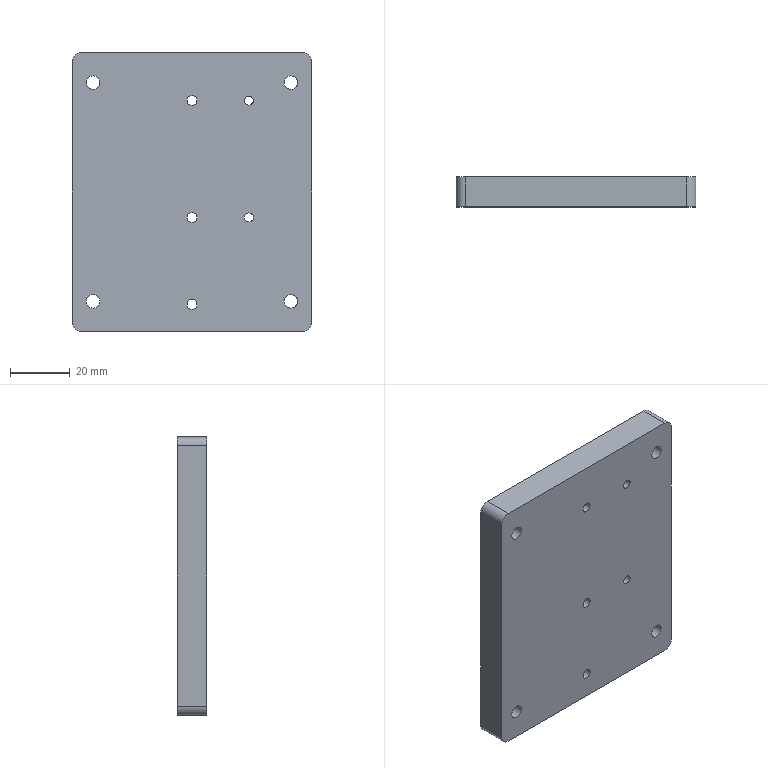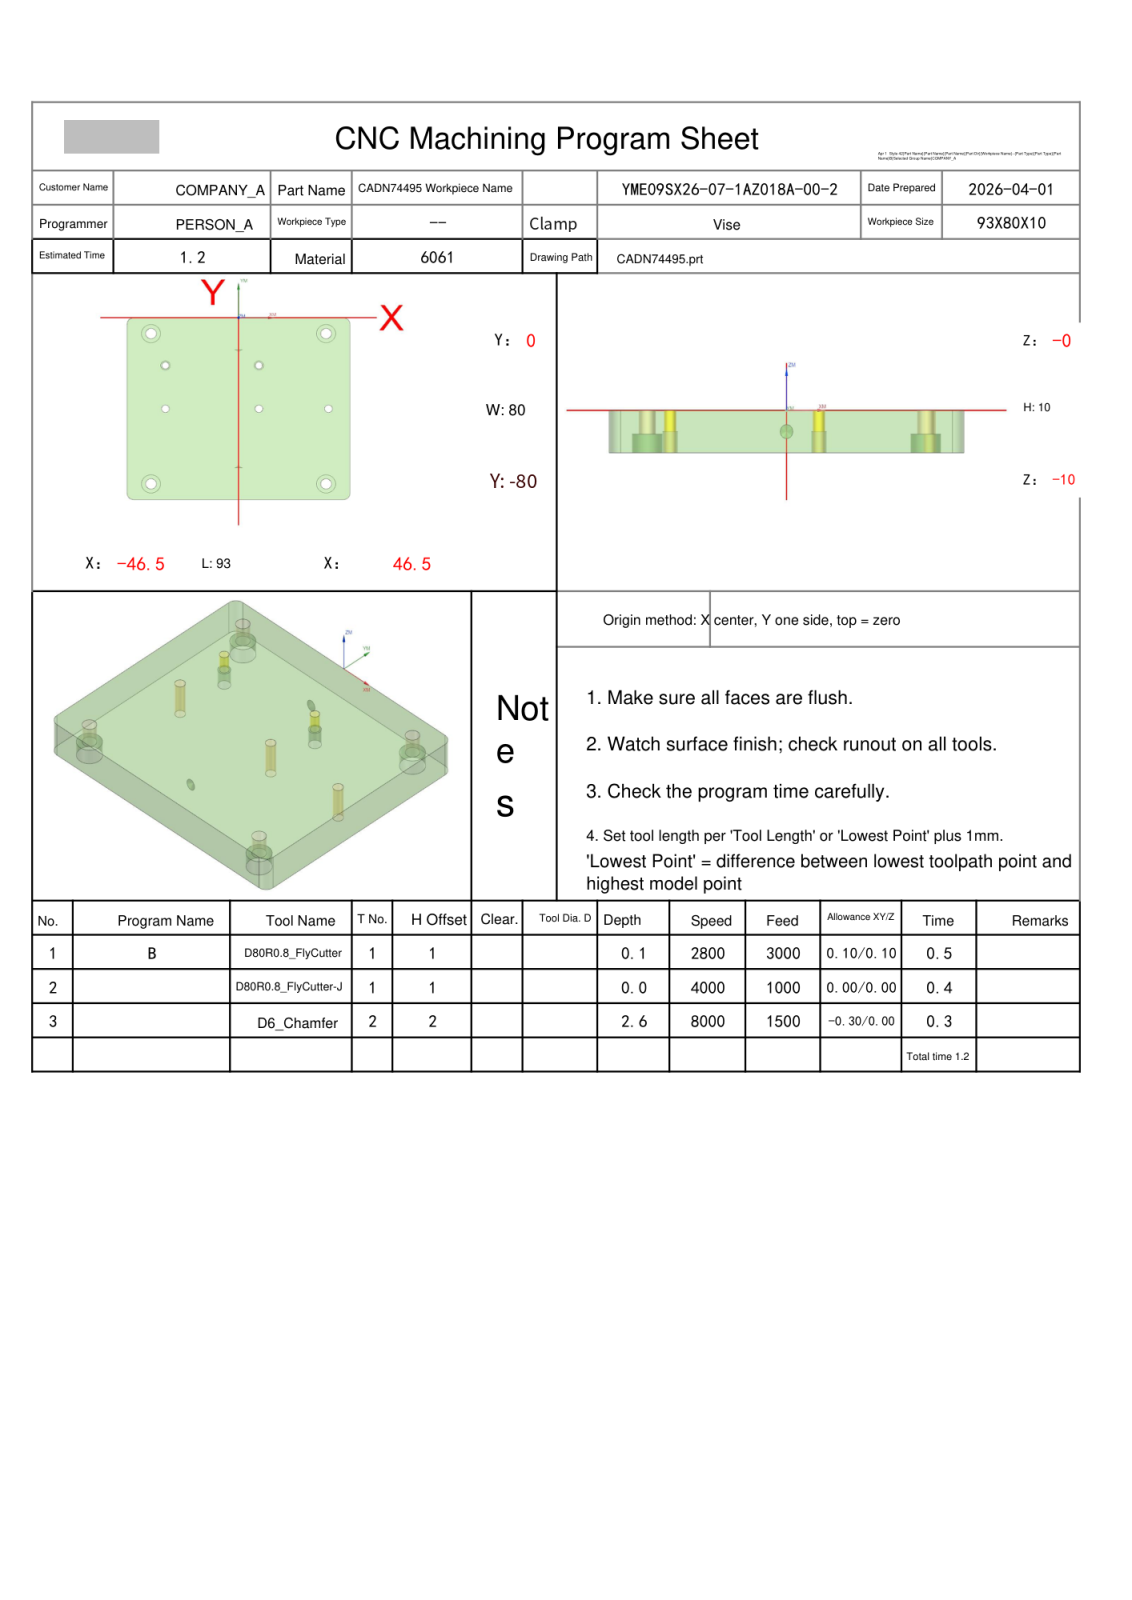NC program | NX | posted by the shop | part box 80 x 10 x 93 mm
Whole program:
%
O0001
(Machine time: 1.87 MIN)
(===Total Tool:2===)
(T1=D80R0.8 FlyCutter D=80.  R=0.8  D-  H01 Z=0.    )
(T2=D6_Chamfer   D=6.   R=0.   D-  H02 Z=-2.55 )
G80 G90 G17 G49 G40
G91 G28 Z0
M01
N1 T01 M06
(D80R0.8 FlyCutter  D=80. R=0.8 H=01 ce=0.10 di=0.10)
G00 G90 G54 X98.597 Y-56.097 M03 S2800
G43 H01 Z20.
M08
Z3.525
G01 Z1.525 F3000.
X86.597
X-79.397
G02 X-86.597 Y-48.897 I0.0 J7.2
G01 Y-39.263
G02 X-78.597 Y-31.263 I8. J0.0
G01 X86.597
X98.597
Z3.525
G00 Y-56.097
Z3.05
G01 Z1.05
X86.597
X-79.397
G02 X-86.597 Y-48.897 I0.0 J7.2
G01 Y-39.263
G02 X-78.597 Y-31.263 I8. J0.0
G01 X86.597
X98.597
Z3.05
G00 Y-56.097
Z2.575
G01 Z.575
X86.597
X-79.397
G02 X-86.597 Y-48.897 I0.0 J7.2
G01 Y-39.263
G02 X-78.597 Y-31.263 I8. J0.0
G01 X86.597
X98.597
Z2.575
G00 Y-56.097
Z2.1
G01 Z.1
X86.597
X-79.397
G02 X-86.597 Y-48.897 I0.0 J7.2
G01 Y-39.263
G02 X-78.597 Y-31.263 I8. J0.0
G01 X86.597
X98.597
Z2.1
G00 Z20.
G91 G28 Z0.0
M05
M09
G91 G28 Z0.0
M01
N2 T01 M06
(D80R0.8 FlyCutter-J  D=80. R=0.8 H=01 ce=0.00 di=0.00)
G00 G90 G54 X98.499 Y-55.999 M03 S4000
G43 H01 Z20.
M08
Z2.
G01 Z0.0 F1000.
X86.499
X-79.299
G02 X-86.499 Y-48.799 I0.0 J7.2
G01 Y-39.361
G02 X-78.499 Y-31.361 I8. J0.0
G01 X86.499
X98.499
Z2.
G00 Z20.
G91 G28 Z0.0
M05
M09
G91 G28 Z0.0
M01
N3 T02 M06
(D6_Chamfer  D=6. R=0. H=02 ce=0.00 di=0.00)
G00 G90 G54 X-30.5 Y-21. M03 S8000
G43 H02 Z20.
M08
G98 G81 X-30.5 Y-21. Z-1.8 R3. F1000.
X8.5
G80
G00 Z20.
G00 G90 X-36.5 Y-73. M03 S8000
Z20.
G98 G81 X-36.5 Y-73. Z-2.55 R3. F1000.
Y-7.
X36.5
Y-73.
G80
G00 Z20.
G00 G90 X37.5 Y-40. M03 S8000
Z20.
G98 G81 X37.5 Y-40. Z-2.2 R3. F1000.
X8.5
X-30.5
G80
G00 Z20.
G00 G90 X33.884 Y.7 M03 S7000
Z20.
Z2.5
G01 X43.5 Z-1. F1500.
G02 X47.2 Y-3. I0.0 J-3.7
G01 Y-77.
G02 X43.5 Y-80.7 I-3.7 J0.0
G01 X-43.5
G02 X-47.2 Y-77. I0.0 J3.7
G01 Y-3.
G02 X-43.5 Y.7 I3.7 J0.0
G01 X43.5
G02 X43.998 Y.666 I0.0 J-3.7
G01 Z1.5
G00 Z20.
M05
M09
G91 G28 Z0.0
G91 G28 Y0.0
M30
%